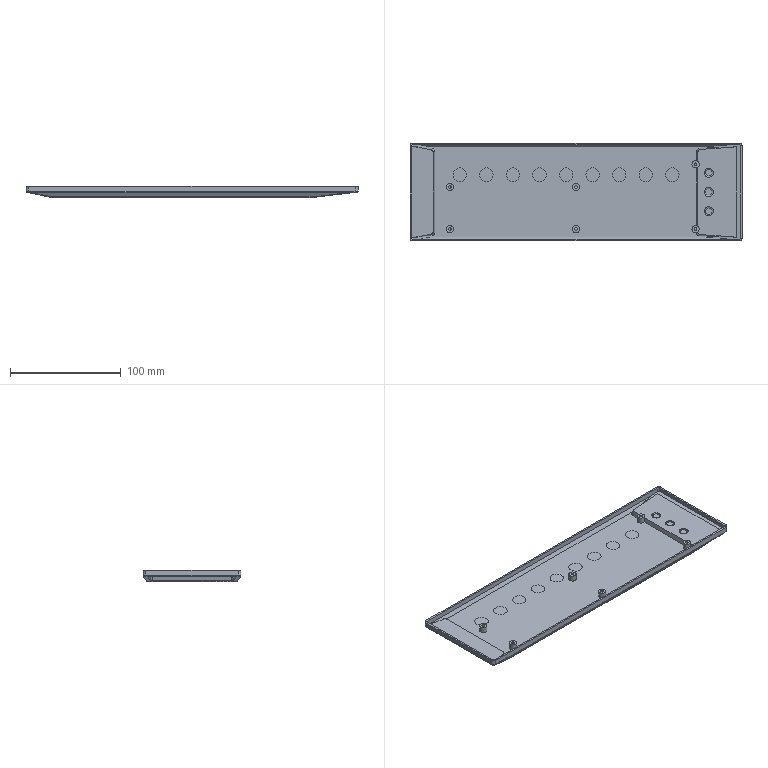NC program | NX | posted with a generic post | part box 300 x 88.5 x 10 mm
Lines 1 to 1164 of 79950:
N10 G17 G21 G94 G90
(FLOOR_WALL_COPY , TOOL : D63)
N12 T01 M6
N14 G54
N16 G17 G0 G90 X-186.5 Y44.247 S6500 M3
N18 G43 Z30. H1
N20 Z4.5
N22 G94 G1 Z1.5 F1250.
N24 X-181.5
N26 X181.5
N28 Y12.599
N30 X-181.5
N32 Y-19.05
N34 X181.5
N36 X186.5
N38 Z4.5
N40 G0 Z30.
N42 X-186.5 Y44.247
N44 Z4.
N46 G1 Z1.
N48 X-181.5
N50 X181.5
N52 Y12.599
N54 X-181.5
N56 Y-19.05
N58 X181.5
N60 X186.5
N62 Z4.
N64 G0 Z30.
N66 X-186.5 Y44.247
N68 Z3.5
N70 G1 Z0.5
N72 X-181.5
N74 X181.5
N76 Y12.599
N78 X-181.5
N80 Y-19.05
N82 X181.5
N84 X186.5
N86 Z3.5
N88 G0 Z30.
N90 X-186.5 Y44.247
N92 Z3.
N94 G1 Z0.
N96 X-181.5
N98 X181.5
N100 Y12.599
N102 X-181.5
N104 Y-19.05
N106 X181.5
N108 X186.5
N110 Z3.
N112 G0 Z30.
N114 M5
(CAVITY_MILL_COPY_1 , TOOL : D8)
N116 T08 M6
N118 G54
N120 G17 G0 G90 X75.78 Y16.213 S9500 M3
N122 G43 Z30. H8
N124 Z1.5
N126 G94 G1 X104.437 Z-0.002 F1000.
N128 Y18.087 Z-0.1
N130 X-86.437 F3000.
N132 Y16.213
N134 X104.437
N136 Y18.087
N138 X109.237
N140 Y22.887
N142 X-91.237
N144 Y11.413
N146 X109.237
N148 Y18.087
N150 X114.037
N152 Y27.687
N154 X-95.959
N156 X-96.037 Y27.632
N158 Y6.828
N160 X-95.762 Y6.613
N162 X114.037
N164 Y18.087
N166 X118.837
N168 Y30.196
N170 X115.905 Y32.487
N172 X-97.476
N174 X-100.837 Y30.127
N176 Y4.486
N178 X-97.415 Y1.813
N180 X115.841
N182 X118.837 Y4.417
N184 Y18.087
N186 G3 X118.48 Y18.853 R1.
N188 G1 Z0.9
N190 G0 Z30.
N192 X70.164 Y16.813
N194 Z1.4
N196 G1 X103.837 Z-0.365 F1000.
N198 Y17.487 Z-0.4
N200 X-85.837 F3000.
N202 Y16.813
N204 X103.837
N206 Y17.487
N208 Y21.087
N210 X-89.437
N212 Y13.213
N214 X107.437
N216 Y21.087
N218 X103.837
N220 Y25.887
N222 X-94.237
N224 Y8.413
N226 X112.237
N228 Y25.887
N230 X103.837
N232 Y30.687
N234 X-96.908
N236 X-99.037 Y29.192
N238 Y5.364
N240 X-96.795 Y3.613
N242 X115.168
N244 X117.037 Y5.238
N246 Y29.318
N248 X115.285 Y30.687
N250 X103.837
N252 G3 X103.071 Y30.33 R1.
N254 G1 Z0.6
N256 G0 Z30.
N258 X65.938 Y16.95
N260 Z1.1
N262 G1 X103.7 Z-0.879 F1000.
N264 Y17.35 Z-0.9
N266 X-85.7 F3000.
N268 Y16.95
N270 X103.7
N272 Y17.35
N274 Y20.95
N276 X-89.3
N278 Y13.35
N280 X107.3
N282 Y20.95
N284 X103.7
N286 Y25.75
N288 X-94.1
N290 Y8.55
N292 X112.1
N294 Y25.75
N296 X103.7
N298 Y30.55
N300 X-96.864
N302 X-98.9 Y29.121
N304 Y5.527
N306 X-98.899 Y5.43
N308 X-96.748 Y3.75
N310 X115.117
N312 X116.9 Y5.3
N314 Y29.252
N316 X115.238 Y30.55
N318 X103.7
N320 G3 X102.934 Y30.193 R1.
N322 G1 Z0.1
N324 G0 Z30.
N326 X-154.203 Y-47.946
N328 Z0.9
N330 G1 Z-0.1 F1000.
N332 X-150.753 Y-45.05
N334 G3 X-150.396 Y-44.284 R1.
N336 G1 Y44.284 F3000.
N338 G2 X-150.029 Y44.646 R0.397
N340 G1 X-113.089
N342 G2 X-108.99 Y46.238 R6.156
N344 X-108.44 Y46.265 R5.582
N346 G1 X126.395
N348 G2 X127.082 Y46.223 R5.582
N350 X130.617 Y44.646 R5.732
N352 G1 X150.029
N354 G2 X150.396 Y44.284 R0.397
N356 G1 Y-44.284
N358 G2 X150.029 Y-44.646 R0.397
N360 G1 X132.375
N362 Y-39.846
N364 Y-38.968
N366 X132.369 Y-38.81
N368 X132.356 Y-38.681
N370 X132.191 Y-37.715
N372 X132.363 Y-36.653
N374 X132.375 Y-36.5
N376 Y-34.
N378 G3 X132.348 Y-33.773 R0.96
N380 G2 X132.276 Y-32.618 R3.305
N382 G1 X132.304 Y-32.374
N384 X132.365 Y-31.814
N386 X132.375 Y-31.5
N388 X132.364 Y-23.686
N390 X132.3 Y-22.976
N392 G2 X132.36 Y-21.633 R5.009
N394 G1 X132.375 Y-21.463
N396 Y-19.
N398 X132.363 Y-18.848
N400 X132.186 Y-17.745
N402 X132.363 Y-16.654
N404 X132.375 Y-16.5
N406 Y-13.978
N408 X132.371 Y-13.796
N410 X132.349 Y-13.607
N412 X132.195 Y-12.735
N414 X132.352 Y-11.916
N416 X132.367 Y-11.774
N418 X132.375 Y-11.5
N420 Y-9.
N422 X132.363 Y-8.849
N424 X132.19 Y-7.762
N426 X132.35 Y-6.885
N428 X132.365 Y-6.754
N430 X132.375 Y-6.5
N432 Y39.846
N434 X145.596
N436 Y-39.846
N438 X132.375
N440 X137.175 Y-35.046
N442 Y-34.
N444 G3 X137.073 Y-32.919 R5.76
N446 G1 X137.128 Y-32.434
N448 G3 X137.162 Y-31.981 R5.76
N450 G1 X137.164 Y-23.466
N452 X137.081 Y-22.544
N454 X137.083 Y-22.488
N456 G3 X137.175 Y-21.463 R5.76
N458 G1 Y-19.
N460 G3 X137.102 Y-18.087 R5.76
N462 G1 X137.048 Y-17.749
N464 X137.101 Y-17.421
N466 G3 X137.175 Y-16.5 R5.76
N468 G1 X137.17 Y-13.687
N470 G3 X137.076 Y-12.772 R5.76
N472 X137.165 Y-11.92 R5.76
N474 G1 X137.174 Y-11.639
N476 X137.175 Y-11.537
N478 Y-9.
N480 G3 X137.103 Y-8.092 R5.76
N482 G1 X137.072 Y-7.75
N484 G3 X137.161 Y-6.962 R5.76
N486 G1 X137.175 Y35.046
N488 X140.796
N490 Y-35.046
N492 X137.175
N494 X132.375 Y-39.846
N496 Y-44.646
N498 X130.601
N500 G2 X127.438 Y-46.167 R5.729
N502 X126.395 Y-46.265 R5.582
N504 G1 X-108.44
N506 G2 X-109.067 Y-46.23 R5.582
N508 X-113.099 Y-44.646 R6.118
N510 G1 X-150.029
N512 G2 X-150.396 Y-44.284 R0.397
N514 G1 X-145.596 Y-39.846
N516 Y39.846
N518 X-115.064
N520 Y-39.846
N522 X-114.104
N524 Y40.795
N526 G2 X-108.94 Y45.278 R5.196
N528 X-108.44 Y45.305 R4.622
N530 G1 X126.395
N532 G2 X126.987 Y45.267 R4.622
N534 X131.415 Y40.785 R4.772
N536 G1 Y-6.5
N538 X131.406 Y-6.712
N540 X131.216 Y-7.751
N542 X131.415 Y-9.
N544 Y-11.5
N546 X131.408 Y-11.745
N548 X131.214 Y-12.751
N550 X131.234 Y-12.816
N552 X131.411 Y-13.817
N554 X131.415 Y-14.
N556 Y-16.5
N558 X131.214 Y-17.745
N560 X131.415 Y-19.
N562 Y-21.463
N564 G3 X131.344 Y-23.062 R5.969
N566 G1 X131.408 Y-23.773
N568 X131.415 Y-24.
N570 Y-31.5
N572 X131.405 Y-31.78
N574 X131.322 Y-32.509
N576 G3 X131.415 Y-34. R4.265
N578 G1 Y-36.5
N580 X131.214 Y-37.746
N582 X131.233 Y-37.809
N584 X131.41 Y-38.843
N586 X131.415 Y-39.
N588 Y-40.785
N590 G2 X127.282 Y-45.219 R4.769
N592 X126.395 Y-45.305 R4.622
N594 G1 X-108.44
N596 G2 X-109.007 Y-45.271 R4.622
N598 X-114.104 Y-40.795 R5.158
N600 G1 Y-39.846
N602 X-115.064
N604 X-145.596
N606 X-140.796 Y-35.046
N608 Y35.046
N610 X-119.864
N612 Y-35.046
N614 X-140.796
N616 X-135.996 Y-30.246
N618 Y30.246
N620 X-124.664
N622 Y-30.246
N624 X-135.996
N626 X-131.196 Y-25.446
N628 Y25.446
N630 X-129.464
N632 Y-25.446
N634 X-131.196
N636 G3 X-131.962 Y-25.803 R1.
N638 G1 Z0.9
N640 G0 Z30.
N642 X-154.203 Y-47.946
N644 Z0.6
N646 G1 Z-0.4 F1000.
N648 X-150.753 Y-45.05
N650 G3 X-150.396 Y-44.284 R1.
N652 G1 Y44.284 F3000.
N654 G2 X-150.029 Y44.646 R0.397
N656 G1 X-115.973
N658 G2 X-113.598 Y45.994 R5.293
N660 X-108.434 Y46.561 R21.468
N662 G1 X126.388
N664 G2 X130.358 Y45.893 R11.221
N666 X132.248 Y44.646 R5.38
N668 G1 X150.029
N670 G2 X150.396 Y44.284 R0.397
N672 G1 Y-44.284
N674 G2 X150.029 Y-44.646 R0.397
N676 G1 X133.785
N678 Y-39.846
N680 Y39.846
N682 X145.596
N684 Y-39.846
N686 X133.785
N688 X138.585 Y-35.046
N690 Y35.046
N692 X140.796
N694 Y-35.046
N696 X138.585
N698 X133.785 Y-39.846
N700 Y-44.646
N702 X132.285
N704 G2 X130.215 Y-45.945 R5.249
N706 X126.392 Y-46.561 R11.735
N708 G1 X-108.434
N710 G2 X-113.625 Y-45.987 R21.27
N712 X-115.973 Y-44.646 R5.293
N714 G1 X-150.029
N716 G2 X-150.396 Y-44.284 R0.397
N718 G1 X-145.596 Y-39.846
N720 Y39.846
N722 X-117.554
N724 Y38.014
N726 G3 X-115.49 Y33.979 R4.988
N728 G1 Y-33.988
N730 G3 X-117.554 Y-38.013 R4.962
N732 G1 Y-39.846
N734 X-116.594
N736 Y-38.014
N738 G2 X-114.53 Y-34.515 R4.002
N740 G1 Y34.503
N742 G2 X-116.594 Y38.014 R4.028
N744 G1 Y40.975
N746 G2 X-113.378 Y45.059 R4.333
N748 X-108.44 Y45.601 R20.508
N750 G1 X126.395
N752 G2 X130.01 Y44.999 R10.261
N754 X132.825 Y40.965 R4.42
N756 G1 Y-40.971
N758 G2 X129.908 Y-45.035 R4.289
N760 X126.395 Y-45.601 R10.775
N762 G1 X-108.44
N764 G2 X-113.378 Y-45.059 R20.31
N766 X-116.594 Y-40.975 R4.333
N768 G1 Y-39.846
N770 X-117.554
N772 X-145.596
N774 X-140.796 Y-35.046
N776 Y35.046
N778 X-121.891
N780 G3 X-120.29 Y32.008 R9.788
N782 G1 Y-32.013
N784 G3 X-121.891 Y-35.046 R9.762
N786 G1 X-140.796
N788 X-135.996 Y-30.246
N790 Y30.246
N792 X-125.09
N794 Y-30.246
N796 X-135.996
N798 X-131.196 Y-25.446
N800 Y25.446
N802 X-129.89
N804 Y-25.446
N806 X-131.196
N808 G3 X-131.962 Y-25.803 R1.
N810 G1 Z0.6
N812 G0 Z30.
N814 X-154.204 Y-47.946
N816 Z0.1
N818 G1 Z-0.9 F1000.
N820 X-150.753 Y-45.05
N822 G3 X-150.396 Y-44.284 R1.
N824 G1 Y44.284 F3000.
N826 G2 X-150.029 Y44.646 R0.397
N828 G1 X-120.388
N830 G2 X-117.263 Y46.439 R5.432
N832 X-112.238 Y46.862 R25.54
N834 G1 X128.553
N836 X129.181 Y46.86
N838 G2 X133.206 Y45.931 R9.35
N840 X134.881 Y44.646 R5.179
N842 G1 X150.029
N844 G2 X150.396 Y44.284 R0.397
N846 G1 Y-44.284
N848 G2 X150.029 Y-44.646 R0.397
N850 G1 X136.135
N852 Y-39.846
N854 Y-37.81
N856 G3 X134.503 Y-34.12 R5.016
N858 G1 Y34.124
N860 G3 X136.135 Y37.81 R5.015
N862 G1 Y39.846
N864 X145.596
N866 Y-39.846
N868 X136.135
N870 X140.534 Y-35.046
N872 G3 X139.303 Y-32.402 R9.816
N874 G1 Y32.406
N876 G3 X140.533 Y35.046 R9.815
N878 G1 X140.796
N880 Y-35.046
N882 X140.534
N884 X136.135 Y-39.846
N886 Y-44.646
N888 X134.853
N890 G2 X131.674 Y-46.54 R5.556
N892 X128.55 Y-46.862 R17.454
N894 G1 X-112.241
N896 G2 X-117.209 Y-46.452 R27.419
N898 X-120.39 Y-44.646 R5.435
N900 G1 X-150.029
N902 G2 X-150.396 Y-44.284 R0.397
N904 G1 X-145.596 Y-39.846
N906 Y39.846
N908 X-121.704
N910 Y38.18
N912 G3 X-116.929 Y33.144 R5.147
N914 G1 X-115.624 Y33.05
N916 Y-33.05
N918 X-116.929 Y-33.144
N920 G3 X-121.704 Y-38.18 R5.147
N922 G1 Y-39.846
N924 X-120.744
N926 Y-38.18
N928 G2 X-116.86 Y-34.101 R4.187
N930 G1 X-114.664 Y-33.943
N932 Y33.943
N934 X-116.86 Y34.101
N936 G2 X-120.744 Y38.18 R4.187
N938 G1 Y41.275
N940 G2 X-117.089 Y45.495 R4.472
N942 X-112.245 Y45.902 R24.58
N944 G1 X128.55
N946 X129.178 Y45.9
N948 G2 X132.789 Y45.067 R8.39
N950 X135.175 Y41.267 R4.219
N952 G1 Y37.81
N954 G2 X133.543 Y34.574 R4.055
N956 G1 Y-34.571
N958 G2 X135.175 Y-37.81 R4.056
N960 G1 Y-41.265
N962 G2 X131.49 Y-45.598 R4.596
N964 X128.55 Y-45.902 R16.494
N966 G1 X-112.245
N968 G2 X-117.044 Y-45.507 R26.459
N970 X-120.744 Y-41.275 R4.475
N972 G1 Y-39.846
N974 X-121.704
N976 X-145.596
N978 X-140.796 Y-35.046
N980 Y35.046
N982 X-125.965
N984 G3 X-120.424 Y29.113 R9.947
N986 G1 Y-29.113
N988 G3 X-125.965 Y-35.046 R9.947
N990 G1 X-140.796
N992 X-135.996 Y-30.246
N994 Y30.246
N996 X-128.926
N998 G3 X-125.224 Y26.345 R14.747
N1000 G1 Y-26.345
N1002 G3 X-128.926 Y-30.246 R14.747
N1004 G1 X-135.996
N1006 X-131.196 Y-25.323
N1008 Y25.323
N1010 G3 X-130.024 Y24.109 R19.547
N1012 G1 Y-24.109
N1014 G3 X-131.196 Y-25.323 R19.547
N1016 X-131.436 Y-26.134 R1.
N1018 G1 Z0.1
N1020 G0 X-154.204 Y-47.946 Z-0.58
N1022 G1 Z-1.58 F1000.
N1024 X-150.753 Y-45.05
N1026 G3 X-150.396 Y-44.284 R1.
N1028 G1 Y44.284 F3000.
N1030 G2 X-150.029 Y44.646 R0.398
N1032 G1 X-126.421
N1034 G2 X-123.219 Y46.78 R5.377
N1036 X-118.78 Y47.275 R20.172
N1038 G1 X132.061
N1040 G2 X136.08 Y46.51 R10.946
N1042 X138.436 Y44.646 R5.193
N1044 G1 X150.029
N1046 G2 X150.396 Y44.284 R0.398
N1048 G1 Y-44.284
N1050 G2 X150.029 Y-44.646 R0.398
N1052 G1 X139.367
N1054 Y-39.846
N1056 Y-38.193
N1058 G3 X134.911 Y-33.171 R5.214
N1060 G1 X134.687 Y-33.131
N1062 Y33.131
N1064 X134.911 Y33.171
N1066 G3 X139.367 Y38.193 R5.214
N1068 G1 Y39.846
N1070 X145.596
N1072 Y-39.846
N1074 X139.367
N1076 X140.796 Y-30.835
N1078 G3 X139.487 Y-29.854 R10.014
N1080 G1 Y29.854
N1082 G3 X140.796 Y30.835 R10.014
N1084 G1 Y-30.835
N1086 X139.367 Y-39.846
N1088 Y-44.646
N1090 X138.449
N1092 G2 X135.754 Y-46.671 R5.254
N1094 X131.772 Y-47.275 R12.083
N1096 G1 X-117.946
N1098 G2 X-123.28 Y-46.766 R25.028
N1100 X-126.421 Y-44.646 R5.377
N1102 G1 X-150.029
N1104 G2 X-150.396 Y-44.284 R0.398
N1106 G1 X-145.596 Y-39.846
N1108 Y39.846
N1110 X-127.41
N1112 Y38.408
N1114 G3 X-123.198 Y33.475 R5.048
N1116 G1 X-122.339 Y33.351
N1118 X-122.194 Y33.34
N1120 X-115.808 Y32.878
N1122 Y-32.878
N1124 X-120.262 Y-33.2
N1126 X-122.201 Y-33.34
N1128 X-122.413 Y-33.359
N1130 X-123.198 Y-33.475
N1132 G3 X-127.41 Y-38.408 R5.048
N1134 G1 Y-39.846
N1136 X-126.45
N1138 Y-38.408
N1140 G2 X-123.058 Y-34.425 R4.088
N1142 G1 X-122.273 Y-34.309
N1144 X-122.124 Y-34.297
N1146 X-114.848 Y-33.771
N1148 Y33.771
N1150 X-122.124 Y34.297
N1152 X-122.263 Y34.308
N1154 X-123.058 Y34.425
N1156 G2 X-126.45 Y38.408 R4.088
N1158 G1 Y41.687
N1160 G2 X-123.007 Y45.844 R4.417
N1162 X-118.78 Y46.315 R19.212
N1164 G1 X132.061
N1166 G2 X135.728 Y45.617 R9.986
N1168 X138.407 Y41.68 R4.233
N1170 G1 Y38.193
N1172 G2 X134.759 Y34.119 R4.254
N1174 G1 X133.727 Y33.937
N1176 Y-33.937
N1178 X134.759 Y-34.119
N1180 G2 X138.407 Y-38.193 R4.254
N1182 G1 Y-41.68
N1184 G2 X135.454 Y-45.759 R4.294
N1186 X131.781 Y-46.315 R11.123
N1188 G1 X-117.951
N1190 G2 X-123.058 Y-45.832 R24.068
N1192 X-126.45 Y-41.687 R4.417
N1194 G1 Y-39.846
N1196 X-127.41
N1198 X-145.596
N1200 X-140.796 Y-35.046
N1202 Y35.046
N1204 X-131.602
N1206 G3 X-123.944 Y28.733 R9.848
N1208 G1 X-123.021 Y28.598
N1210 X-122.798 Y28.573
N1212 X-122.548 Y28.553
N1214 X-120.608 Y28.413
N1216 Y-28.413
N1218 X-122.573 Y-28.555
N1220 X-122.811 Y-28.574
N1222 X-123.035 Y-28.599
N1224 X-123.993 Y-28.742
N1226 G3 X-131.602 Y-35.046 R9.848
N1228 G1 X-140.796
N1230 X-135.996 Y-30.246
N1232 Y30.246
N1234 X-134.495
N1236 G3 X-125.408 Y24.126 R14.648
N1238 G1 Y-24.126
N1240 G3 X-134.495 Y-30.246 R14.648
N1242 G1 X-135.996
N1244 X-131.196 Y-21.128
N1246 Y21.128
N1248 G3 X-130.208 Y20.658 R19.448
N1250 G1 Y-20.658
N1252 G3 X-131.196 Y-21.128 R19.448
N1254 X-131.716 Y-21.794 R1.
N1256 G1 Z-0.58
N1258 G0 X-154.204 Y-47.946 Z-1.26
N1260 G1 Z-2.26 F1000.
N1262 X-150.754 Y-45.05
N1264 G3 X-150.396 Y-44.284 R1.
N1266 G1 Y44.284 F3000.
N1268 G2 X-150.029 Y44.646 R0.398
N1270 G1 X-132.309
N1272 G2 X-128.533 Y47.277 R5.484
N1274 X-123.59 Y47.683 R26.496
N1276 G1 X134.973
N1278 G2 X138.57 Y47.222 R13.461
N1280 X141.848 Y44.646 R5.503
N1282 G1 X150.029
N1284 G2 X150.396 Y44.284 R0.398
N1286 G1 Y-44.284
N1288 G2 X150.029 Y-44.646 R0.398
N1290 G1 X142.563
N1292 Y-39.846
N1294 Y-38.572
N1296 G3 X138.111 Y-33.55 R5.255
N1298 G1 X134.87 Y-32.978
N1300 Y32.978
N1302 X138.111 Y33.55
N1304 G3 X142.563 Y38.572 R5.255
N1306 G1 Y39.846
N1308 X145.596
N1310 Y-39.846
N1312 X142.563
N1314 X140.796 Y-29.312
N1316 G3 X139.67 Y-28.969 R10.055
N1318 G1 Y28.969
N1320 G3 X140.796 Y29.312 R10.055
N1322 G1 Y-29.312
N1324 X142.563 Y-39.846
N1326 Y-44.646
N1328 X141.859
N1330 G2 X138.556 Y-47.226 R5.458
N1332 X134.973 Y-47.683 R13.375
N1334 G1 X-123.59
N1336 G2 X-128.526 Y-47.278 R26.804
N1338 X-132.309 Y-44.646 R5.484
N1340 G1 X-150.029
N1342 G2 X-150.396 Y-44.284 R0.398
N1344 G1 X-145.596 Y-39.846
N1346 Y39.846
N1348 X-133.054
N1350 Y38.633
N1352 G3 X-128.285 Y33.597 R5.141
N1354 G1 X-115.99 Y32.709
N1356 Y-32.709
N1358 X-128.283 Y-33.597
N1360 G3 X-133.054 Y-38.633 R5.142
N1362 G1 Y-39.846
N1364 X-132.094
N1366 Y-38.633
N1368 G2 X-128.214 Y-34.555 R4.182
N1370 G1 X-115.03 Y-33.602
N1372 Y33.602
N1374 X-128.215 Y34.555
N1376 G2 X-132.094 Y38.633 R4.181
N1378 G1 Y42.095
N1380 G2 X-128.365 Y46.332 R4.524
N1382 X-123.595 Y46.723 R25.536
N1384 G1 X134.977
N1386 G2 X138.307 Y46.299 R12.501
N1388 X141.603 Y42.085 R4.543
N1390 G1 Y38.572
N1392 G2 X137.955 Y34.497 R4.295
N1394 G1 X133.91 Y33.784
N1396 Y-33.784
N1398 X137.955 Y-34.497
N1400 G2 X141.603 Y-38.572 R4.295
N1402 G1 Y-42.085
N1404 G2 X138.307 Y-46.299 R4.498
N1406 X134.977 Y-46.723 R12.415
N1408 G1 X-123.595
N1410 G2 X-128.36 Y-46.333 R25.844
N1412 X-132.094 Y-42.095 R4.524
N1414 G1 Y-39.846
N1416 X-133.054
N1418 X-145.596
N1420 X-140.796 Y-35.046
N1422 Y35.046
N1424 X-137.149
N1426 G3 X-128.631 Y28.81 R9.941
N1428 G1 X-120.79 Y28.243
N1430 Y-28.243
N1432 X-128.63 Y-28.81
N1434 G3 X-137.149 Y-35.046 R9.942
N1436 G1 X-140.796
N1438 X-135.996 Y-26.398
N1440 Y26.397
N1442 G3 X-128.977 Y24.022 R14.741
N1444 G1 X-125.59 Y23.778
N1446 Y-23.778
N1448 X-128.976 Y-24.022
N1450 G3 X-135.996 Y-26.398 R14.742
N1452 G1 X-131.196 Y-19.462
N1454 Y19.462
N1456 G3 X-130.39 Y19.342 R19.541
N1458 G1 Y-19.342
N1460 G3 X-131.196 Y-19.462 R19.542
N1462 X-131.891 Y-19.943 R1.
N1464 G1 Z-1.26
N1466 G0 X-154.204 Y-47.946 Z-1.94
N1468 G1 Z-2.94 F1000.
N1470 X-150.754 Y-45.05
N1472 G3 X-150.396 Y-44.284 R1.
N1474 G1 Y44.284 F3000.
N1476 G2 X-150.029 Y44.647 R0.398
N1478 G1 X-138.178
N1480 G2 X-134.301 Y47.649 R5.425
N1482 X-129.232 Y48.091 R25.03
N1484 G1 X138.169
N1486 G2 X141.63 Y47.664 R13.464
N1488 X145.251 Y44.647 R5.507
N1490 G1 X150.029
N1492 G2 X150.396 Y44.284 R0.398
N1494 G1 Y-37.814
N1496 X145.596
N1498 G3 X141.307 Y-33.928 R5.256
N1500 G1 X135.052 Y-32.825
N1502 Y32.825
N1504 X141.307 Y33.928
N1506 G3 X145.596 Y37.814 R5.255
N1508 G1 Y-37.814
N1510 X140.796 Y-28.964
N1512 X139.852 Y-28.798
N1514 Y28.798
N1516 X140.796 Y28.964
N1518 Y-28.964
N1520 X145.596 Y-37.814
N1522 X150.396
N1524 Y-44.284
N1526 G2 X150.029 Y-44.647 R0.398
N1528 G1 X145.277
N1530 G2 X142.064 Y-47.487 R5.295
N1532 X138.162 Y-48.091 R11.349
N1534 G1 X-129.234
N1536 G2 X-134.302 Y-47.647 R25.747
N1538 X-138.179 Y-44.647 R5.418
N1540 G1 X-150.029
N1542 G2 X-150.396 Y-44.284 R0.398
N1544 G1 X-145.596 Y-39.847
N1546 Y39.847
N1548 X-138.698
N1550 Y38.858
N1552 G3 X-134.242 Y33.893 R5.044
N1554 G1 X-133.482 Y33.79
N1556 X-116.172 Y32.539
N1558 Y-32.539
N1560 X-120.626 Y-32.861
N1562 X-133.543 Y-33.797
N1564 X-134.242 Y-33.893
N1566 G3 X-138.698 Y-38.848 R5.044
N1568 G1 Y-39.847
N1570 X-137.738
N1572 Y-38.858
N1574 G2 X-134.121 Y-34.845 R4.084
N1576 G1 X-133.412 Y-34.748
N1578 X-115.212 Y-33.432
N1580 Y33.432
N1582 X-133.412 Y34.748
N1584 X-134.121 Y34.845
N1586 G2 X-137.738 Y38.858 R4.084
N1588 G1 Y42.503
N1590 G2 X-134.121 Y46.706 R4.465
N1592 X-129.239 Y47.131 R24.07
N1594 G1 X138.173
N1596 G2 X141.39 Y46.734 R12.504
N1598 X144.799 Y42.493 R4.547
N1600 G1 Y38.95
N1602 G2 X141.151 Y34.876 R4.295
N1604 G1 X134.092 Y33.631
N1606 Y-33.631
N1608 X141.151 Y-34.876
N1610 G2 X144.799 Y-38.95 R4.296
N1612 G1 Y-42.493
N1614 G2 X141.764 Y-46.575 R4.335
N1616 X138.173 Y-47.131 R10.389
N1618 G1 X-129.239
N1620 G2 X-134.121 Y-46.704 R24.787
N1622 X-137.738 Y-42.503 R4.458
N1624 G1 Y-39.847
N1626 X-138.698
N1628 X-145.596
N1630 X-140.796 Y-32.128
N1632 Y32.128
N1634 G3 X-134.855 Y29.132 R9.844
N1636 G1 X-134.118 Y29.031
N1638 X-133.904 Y29.008
N1640 X-120.972 Y28.074
N1642 Y-28.074
N1644 X-133.904 Y-29.008
N1646 X-134.118 Y-29.031
N1648 X-134.855 Y-29.132
N1650 G3 X-140.796 Y-32.128 R9.844
N1652 G1 X-135.996 Y-24.447
N1654 Y24.447
N1656 G3 X-135.477 Y24.372 R14.644
N1658 G1 X-134.693 Y24.265
N1660 X-134.327 Y24.227
N1662 X-125.772 Y23.608
N1664 Y-23.608
N1666 X-134.327 Y-24.227
N1668 X-134.694 Y-24.265
N1670 X-135.477 Y-24.372
N1672 G3 X-135.996 Y-24.447 R14.644
N1674 G1 X-131.196 Y-19.188
N1676 Y19.188
N1678 X-130.572 Y19.143
N1680 Y-19.143
N1682 X-131.196 Y-19.188
N1684 G3 X-131.935 Y-19.599 R1.
N1686 G1 Z-1.94
N1688 G0 X-154.205 Y-47.946 Z-2.62
N1690 G1 Z-3.62 F1000.
N1692 X-150.754 Y-45.05
N1694 G3 X-150.397 Y-44.284 R1.
N1696 G1 Y44.284 F3000.
N1698 G2 X-150.029 Y44.647 R0.398
N1700 G1 X-143.99
N1702 G2 X-139.82 Y48.073 R5.442
N1704 X-138.751 Y48.247 R25.767
N1706 G1 X144.024
N1708 G2 X144.765 Y48.077 R13.109
N1710 X148.613 Y44.647 R5.506
N1712 G1 X150.029
N1714 G2 X150.397 Y44.284 R0.398
N1716 G1 Y-34.592
N1718 X145.597
N1720 G3 X144.499 Y-34.306 R5.214
N1722 G1 X135.234 Y-32.673
N1724 Y32.673
N1726 X144.499 Y34.306
N1728 G3 X145.597 Y34.592 R5.214
N1730 G1 Y-34.592
N1732 X140.797 Y-28.779
N1734 X140.034 Y-28.645
N1736 Y28.645
N1738 X140.797 Y28.779
N1740 Y-28.779
N1742 X145.597 Y-34.592
N1744 X150.397
N1746 Y-44.284
N1748 G2 X150.029 Y-44.647 R0.398
N1750 G1 X148.625
N1752 G2 X144.755 Y-48.092 R5.469
N1754 X144.039 Y-48.247 R14.311
N1756 G1 X-138.723
N1758 G2 X-139.819 Y-48.071 R26.435
N1760 X-143.99 Y-44.647 R5.436
N1762 G1 X-150.029
N1764 G2 X-150.397 Y-44.284 R0.398
N1766 G1 X-145.597 Y-39.847
N1768 Y39.847
N1770 X-144.342
N1772 Y39.078
N1774 G3 X-140.051 Y34.144 R4.982
N1776 G1 X-139.315 Y34.031
N1778 X-139.126 Y34.016
N1780 X-116.355 Y32.37
N1782 Y-32.37
N1784 X-120.808 Y-32.692
N1786 X-139.133 Y-34.016
N1788 X-139.348 Y-34.036
N1790 X-139.826 Y-34.11
N1792 X-139.931 Y-34.129
N1794 X-140.59 Y-34.253
N1796 G3 X-144.342 Y-39.073 R5.045
N1798 G1 Y-39.847
N1800 X-143.382
N1802 Y-39.083
N1804 G2 X-140.344 Y-35.181 R4.085
N1806 G1 X-139.653 Y-35.054
N1808 X-139.202 Y-34.985
N1810 X-139.056 Y-34.973
N1812 X-115.395 Y-33.263
N1814 Y33.263
N1816 X-139.056 Y34.973
N1818 X-139.237 Y34.988
N1820 X-139.986 Y35.106
N1822 G2 X-143.382 Y39.078 R4.021
N1824 G1 Y42.911
N1826 G2 X-139.653 Y47.128 R4.482
N1828 X-134.883 Y47.539 R24.807
N1830 G1 X141.369
N1832 G2 X144.53 Y47.146 R12.149
N1834 X147.995 Y42.901 R4.546
N1836 G1 Y39.329
N1838 G2 X144.347 Y35.254 R4.254
N1840 G1 X134.274 Y33.478
N1842 Y-33.478
N1844 X144.347 Y-35.254
N1846 G2 X147.995 Y-39.329 R4.254
N1848 G1 Y-42.901
N1850 G2 X144.53 Y-47.159 R4.509
N1852 X141.369 Y-47.539 R13.351
N1854 G1 X-134.883
N1856 G2 X-139.653 Y-47.125 R25.475
N1858 X-143.382 Y-42.911 R4.476
N1860 G1 Y-39.847
N1862 X-144.342
N1864 X-145.597
N1866 X-140.797 Y-29.408
N1868 Y29.402
N1870 X-140.133 Y29.298
N1872 G3 X-139.705 Y29.247 R5.76
N1874 G1 X-121.155 Y27.904
N1876 Y-27.904
N1878 X-139.505 Y-29.231
N1880 X-139.659 Y-29.243
N1882 G3 X-140.08 Y-29.292 R5.76
N1884 G1 X-140.564 Y-29.367
N1886 X-140.658 Y-29.383
N1888 X-140.797 Y-29.408
N1890 X-135.997 Y-24.165
N1892 Y24.166
N1894 X-125.955 Y23.439
N1896 Y-23.439
N1898 X-135.997 Y-24.165
N1900 X-131.197 Y-19.005
N1902 Y19.006
N1904 X-130.755 Y18.974
N1906 Y-18.973
N1908 X-131.197 Y-19.005
N1910 G3 X-131.935 Y-19.417 R1.
N1912 G1 Z-2.62
N1914 G0 X-154.205 Y-47.946 Z-3.3
N1916 G1 Z-4.3 F1000.
N1918 X-150.754 Y-45.05
N1920 G3 X-150.397 Y-44.284 R1.
N1922 G1 Y34.32 F3000.
N1924 X-145.597
N1926 G3 X-145.178 Y34.273 R5.115
N1928 G1 X-116.535 Y32.202
N1930 Y-32.202
N1932 X-145.178 Y-34.273
N1934 G3 X-145.597 Y-34.32 R5.115
N1936 G1 Y34.32
N1938 X-140.797 Y29.143
N1940 X-121.335 Y27.736
N1942 Y-27.736
N1944 X-140.797 Y-29.143
N1946 Y29.143
N1948 X-135.997 Y23.984
N1950 X-126.135 Y23.271
N1952 Y-23.271
N1954 X-135.997 Y-23.984
N1956 Y23.984
N1958 X-131.197 Y18.824
N1960 X-130.935 Y18.805
N1962 Y-18.805
N1964 X-131.197 Y-18.824
N1966 Y18.824
N1968 X-140.797 Y29.143
N1970 X-145.597 Y34.32
N1972 X-150.397
N1974 Y44.284
N1976 G2 X-150.029 Y44.647 R0.399
N1978 G1 X-149.665
N1980 G2 X-146.28 Y48.247 R5.73
N1982 G1 X147.694
N1984 G2 X149.042 Y48.064 R6.5
N1986 X152.115 Y43.25 R5.53
N1988 G1 Y39.666
N1990 G2 X150.397 Y35.981 R5.244
N1992 G1 Y-34.317
N1994 X145.597
N1996 X135.414 Y-32.521
N1998 Y32.521
N2000 X145.597 Y34.317
N2002 X145.43 Y35.262
N2004 X134.454 Y33.327
N2006 Y-33.327
N2008 X147.508 Y-35.629
N2010 G2 X151.155 Y-39.703 R4.254
N2012 G1 Y-43.25
N2014 G2 X147.27 Y-47.685 R4.743
N2016 G1 X146.604 Y-47.806
N2018 X144.53 Y-47.942
N2020 X-140.465
N2022 G2 X-144.366 Y-47.72 R50.942
N2024 X-145.058 Y-47.599 R4.491
N2026 X-148.964 Y-43.25 R4.77
N2028 G1 Y-39.306
N2030 G2 X-145.109 Y-35.23 R4.155
N2032 G1 X-115.575 Y-33.095
N2034 Y33.095
N2036 X-145.109 Y35.23
N2038 G2 X-148.964 Y39.306 R4.155
N2040 G1 Y43.25
N2042 G2 X-145.06 Y47.599 R4.77
N2044 X-144.468 Y47.709 R4.491
N2046 X-140.529 Y47.942 R33.454
N2048 G1 X144.53
N2050 G2 X147.987 Y47.46 R11.244
N2052 X151.155 Y43.25 R4.57
N2054 G1 Y39.703
N2056 G2 X147.508 Y35.629 R4.284
N2058 G1 X145.43 Y35.262
N2060 X145.597 Y34.317
N2062 Y-34.317
N2064 X140.797 Y-28.596
N2066 X140.214 Y-28.494
N2068 Y28.494
N2070 X140.797 Y28.596
N2072 Y-28.596
N2074 X145.597 Y-34.317
N2076 X150.397
N2078 Y-35.969
N2080 G2 X152.115 Y-39.703 R5.214
N2082 G1 X152.114 Y-43.297
N2084 G2 X149.106 Y-48.048 R5.703
N2086 X147.694 Y-48.247 R6.5
N2088 G1 X-146.28
N2090 G2 X-149.665 Y-44.647 R5.73
N2092 G1 X-150.029
N2094 G2 X-150.397 Y-44.284 R0.399
N2096 G3 X-150.82 Y-43.552 R1.
N2098 G1 X-155.597 Y-40.209
N2100 Z-3.3
N2102 G0 Z30.
N2104 X155.597 Y35.273
N2106 Z-3.75
N2108 G1 Z-4.75 F1000.
N2110 X150.444
N2112 G3 X150.397 Y35.062 R0.5
N2114 G1 Y-34.194 F3000.
N2116 X145.597
N2118 X135.535 Y-32.42
N2120 Y32.42
N2122 X145.597 Y34.194
N2124 X145.43 Y35.14
N2126 X134.575 Y33.226
N2128 Y-33.226
N2130 X149.843 Y-35.918
N2132 G2 X153.267 Y-39.952 R4.144
N2134 G1 Y-42.048
N2136 G2 X148.857 Y-47.834 R6.002
N2138 X147.02 Y-48.184 R11.609
N2140 X146.497 Y-48.211 R4.961
N2142 G1 X-143.939
N2144 G2 X-144.275 Y-48.2 R4.961
N2146 X-148.642 Y-47.613 R29.376
N2148 X-152.699 Y-42.802 R5.292
N2150 G1 Y42.803
N2152 G2 X-148.642 Y47.613 R5.258
N2154 X-144.275 Y48.2 R29.383
N2156 X-143.939 Y48.211 R4.961
N2158 G1 X146.497
N2160 G2 X147.089 Y48.176 R4.961
N2162 X149.394 Y47.655 R8.829
N2164 X153.238 Y42.38 R5.914
N2166 G1 X153.267 Y41.75
N2168 Y39.952
N2170 G2 X149.623 Y35.879 R4.251
N2172 G1 X145.43 Y35.14
N2174 X145.597 Y34.194
N2176 Y-34.194
N2178 X140.797 Y-28.474
N2180 X140.335 Y-28.392
N2182 Y28.392
N2184 X140.797 Y28.474
N2186 Y-28.474
N2188 X145.597 Y-34.194
N2190 X150.397
N2192 Y-35.056
N2194 G2 X153.997 Y-38.483 R5.104
N2196 G1 Y-41.947
N2198 G2 X147.689 Y-48.247 R6.5
N2200 G1 X-147.689
N2202 G2 X-153.143 Y-44.977 R6.5
N2204 X-153.659 Y-42.802 R6.252
N2206 G1 X-153.657 Y42.86
N2208 G2 X-153.172 Y44.924 R6.218
N2210 X-147.689 Y48.247 R6.5
N2212 G1 X147.689
N2214 G2 X153.997 Y41.947 R6.5
N2216 G1 Y38.549
N2218 G2 X150.397 Y35.062 R5.211
N2220 G3 X149.753 Y34.514 R1.
N2222 G1 X155.597
N2224 Z-3.75
N2226 G0 Z30.
N2228 X-151.153 Y49.728
N2230 Z-3.8
N2232 G1 Z-4.8 F1000.
N2234 X-149.077 Y47.989
N2236 G3 X-148.26 Y47.771 R1.
N2238 G2 X-144.237 Y48.229 R32.469 F3000.
N2240 X-143.939 Y48.238 R4.988
N2242 G1 X146.497
N2244 G2 X147.024 Y48.21 R4.988
N2246 X150.061 Y47.434 R8.635
N2248 X153.419 Y41.75 R6.37
N2250 G1 Y-41.75
N2252 G2 X149.539 Y-47.67 R6.306
N2254 X147.023 Y-48.21 R10.097
N2256 X146.497 Y-48.238 R4.988
N2258 G1 X-143.939
N2260 G2 X-148.277 Y-47.769 R31.572
N2262 X-153.114 Y-41.992 R5.869
N2264 G1 Y41.981
N2266 G2 X-148.26 Y47.771 R5.88
N2268 G3 X-147.568 Y48.257 R1.
N2270 G1 X-146.652 Y49.847
N2272 Z-3.8
N2274 G0 Z30.
N2276 X19.83 Y-25.1
N2278 Z1.5
N2280 G1 X-4.9 Z0.204 F1000.
N2282 Y-30.9 Z-0.1
N2284 X94.9 F3000.
N2286 Y-25.1
N2288 X-4.9
N2290 Y-30.9
N2292 G3 X-4.134 Y-30.543 R1.
N2294 G1 Z0.9
N2296 G0 Z30.
N2298 X23.647 Y-25.1
N2300 Z1.4
N2302 G1 X-4.9 Y-25.101 Z-0.096 F1000.
N2304 Y-30.9 Z-0.4
N2306 X94.9 F3000.
N2308 X94.899 Y-25.1
N2310 X-4.9 Y-25.101
N2312 Y-30.9
N2314 G3 X-4.134 Y-30.543 R1.
N2316 G1 Z0.6
N2318 G0 Z30.
N2320 M5